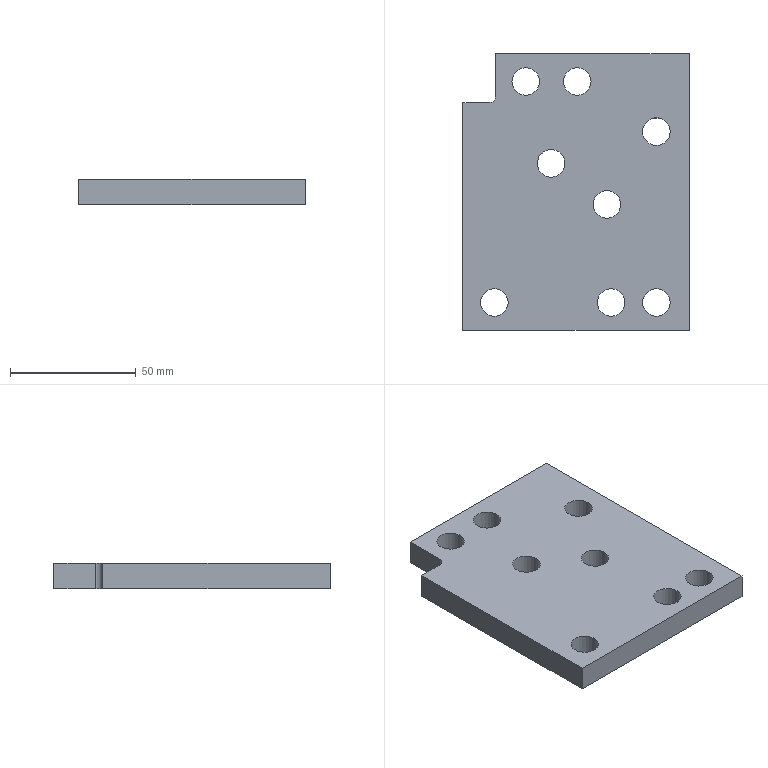Part | NX | features solid 2 | 1 solid | 17 faces | box 90 x 110 x 10 mm | volume 88862 mm3 | cylinder 9 | plane 8 | commonest cylinder face diameters 11 x8 6 x1
STEP:
#1=CARTESIAN_POINT('',(218.5,-15.984,78.));
#2=VERTEX_POINT('',#1);
#3=CARTESIAN_POINT('',(295.411,-15.984,78.));
#4=VERTEX_POINT('',#3);
#5=CARTESIAN_POINT('',(247.131,-15.984,78.));
#6=DIRECTION('',(1.,0.,0.));
#7=VECTOR('',#6,1000.);
#8=LINE('',#5,#7);
#9=EDGE_CURVE('',#2,#4,#8,.T.);
#10=ORIENTED_EDGE('',*,*,#9,.T.);
#11=CARTESIAN_POINT('',(295.411,-125.984,78.));
#12=VERTEX_POINT('',#11);
#13=CARTESIAN_POINT('',(295.411,-71.771,78.));
#14=DIRECTION('',(0.,-1.,0.));
#15=VECTOR('',#14,1000.);
#16=LINE('',#13,#15);
#17=EDGE_CURVE('',#4,#12,#16,.T.);
#18=ORIENTED_EDGE('',*,*,#17,.T.);
#19=CARTESIAN_POINT('',(205.411,-125.984,78.));
#20=VERTEX_POINT('',#19);
#21=CARTESIAN_POINT('',(247.131,-125.984,78.));
#22=DIRECTION('',(-1.,0.,0.));
#23=VECTOR('',#22,1000.);
#24=LINE('',#21,#23);
#25=EDGE_CURVE('',#12,#20,#24,.T.);
#26=ORIENTED_EDGE('',*,*,#25,.T.);
#27=CARTESIAN_POINT('',(205.411,-35.5,78.));
#28=VERTEX_POINT('',#27);
#29=CARTESIAN_POINT('',(205.411,-71.771,78.));
#30=DIRECTION('',(0.,1.,0.));
#31=VECTOR('',#30,1000.);
#32=LINE('',#29,#31);
#33=EDGE_CURVE('',#20,#28,#32,.T.);
#34=ORIENTED_EDGE('',*,*,#33,.T.);
#35=CARTESIAN_POINT('',(215.5,-35.5,78.));
#36=VERTEX_POINT('',#35);
#37=CARTESIAN_POINT('',(188.,-35.5,78.));
#38=DIRECTION('',(-1.,0.,0.));
#39=VECTOR('',#38,1000.);
#40=LINE('',#37,#39);
#41=EDGE_CURVE('',#28,#36,#40,.F.);
#42=ORIENTED_EDGE('',*,*,#41,.T.);
#43=CARTESIAN_POINT('',(218.5,-32.5,78.));
#44=VERTEX_POINT('',#43);
#45=CARTESIAN_POINT('',(215.5,-32.5,78.));
#46=DIRECTION('',(0.,0.,-1.));
#47=DIRECTION('',(-1.,0.,0.));
#48=AXIS2_PLACEMENT_3D('',#45,#46,#47);
#49=CIRCLE('',#48,3.);
#50=EDGE_CURVE('',#36,#44,#49,.F.);
#51=ORIENTED_EDGE('',*,*,#50,.T.);
#52=CARTESIAN_POINT('',(218.5,0.,78.));
#53=DIRECTION('',(0.,-1.,0.));
#54=VECTOR('',#53,1000.);
#55=LINE('',#52,#54);
#56=EDGE_CURVE('',#44,#2,#55,.F.);
#57=ORIENTED_EDGE('',*,*,#56,.T.);
#58=EDGE_LOOP('',(#10,#18,#26,#34,#42,#51,#57));
#59=FACE_BOUND('',#58,.T.);
#60=CARTESIAN_POINT('',(258.911,-114.984,78.));
#61=VERTEX_POINT('',#60);
#62=CARTESIAN_POINT('',(264.411,-114.984,78.));
#63=DIRECTION('',(0.,0.,1.));
#64=DIRECTION('',(-1.,0.,0.));
#65=AXIS2_PLACEMENT_3D('',#62,#63,#64);
#66=CIRCLE('',#65,5.5);
#67=EDGE_CURVE('',#61,#61,#66,.F.);
#68=ORIENTED_EDGE('',*,*,#67,.F.);
#69=EDGE_LOOP('',(#68));
#70=FACE_BOUND('',#69,.T.);
#71=CARTESIAN_POINT('',(276.911,-114.984,78.));
#72=VERTEX_POINT('',#71);
#73=CARTESIAN_POINT('',(282.411,-114.984,78.));
#74=DIRECTION('',(0.,0.,-1.));
#75=DIRECTION('',(-1.,0.,0.));
#76=AXIS2_PLACEMENT_3D('',#73,#74,#75);
#77=CIRCLE('',#76,5.5);
#78=EDGE_CURVE('',#72,#72,#77,.F.);
#79=ORIENTED_EDGE('',*,*,#78,.T.);
#80=EDGE_LOOP('',(#79));
#81=FACE_BOUND('',#80,.T.);
#82=CARTESIAN_POINT('',(224.911,-26.984,78.));
#83=VERTEX_POINT('',#82);
#84=CARTESIAN_POINT('',(230.411,-26.984,78.));
#85=DIRECTION('',(0.,0.,-1.));
#86=DIRECTION('',(-1.,0.,0.));
#87=AXIS2_PLACEMENT_3D('',#84,#85,#86);
#88=CIRCLE('',#87,5.5);
#89=EDGE_CURVE('',#83,#83,#88,.F.);
#90=ORIENTED_EDGE('',*,*,#89,.T.);
#91=EDGE_LOOP('',(#90));
#92=FACE_BOUND('',#91,.T.);
#93=CARTESIAN_POINT('',(276.911,-46.984,78.));
#94=VERTEX_POINT('',#93);
#95=CARTESIAN_POINT('',(282.411,-46.984,78.));
#96=DIRECTION('',(0.,0.,-1.));
#97=DIRECTION('',(-1.,0.,0.));
#98=AXIS2_PLACEMENT_3D('',#95,#96,#97);
#99=CIRCLE('',#98,5.5);
#100=EDGE_CURVE('',#94,#94,#99,.F.);
#101=ORIENTED_EDGE('',*,*,#100,.T.);
#102=EDGE_LOOP('',(#101));
#103=FACE_BOUND('',#102,.T.);
#104=CARTESIAN_POINT('',(212.411,-114.984,78.));
#105=VERTEX_POINT('',#104);
#106=CARTESIAN_POINT('',(217.911,-114.984,78.));
#107=DIRECTION('',(0.,0.,-1.));
#108=DIRECTION('',(-1.,0.,0.));
#109=AXIS2_PLACEMENT_3D('',#106,#107,#108);
#110=CIRCLE('',#109,5.5);
#111=EDGE_CURVE('',#105,#105,#110,.F.);
#112=ORIENTED_EDGE('',*,*,#111,.T.);
#113=EDGE_LOOP('',(#112));
#114=FACE_BOUND('',#113,.T.);
#115=CARTESIAN_POINT('',(245.411,-26.984,78.));
#116=VERTEX_POINT('',#115);
#117=CARTESIAN_POINT('',(250.911,-26.984,78.));
#118=DIRECTION('',(0.,0.,1.));
#119=DIRECTION('',(-1.,0.,0.));
#120=AXIS2_PLACEMENT_3D('',#117,#118,#119);
#121=CIRCLE('',#120,5.5);
#122=EDGE_CURVE('',#116,#116,#121,.T.);
#123=ORIENTED_EDGE('',*,*,#122,.T.);
#124=EDGE_LOOP('',(#123));
#125=FACE_BOUND('',#124,.T.);
#126=CARTESIAN_POINT('',(257.24,-75.929,78.));
#127=VERTEX_POINT('',#126);
#128=CARTESIAN_POINT('',(262.74,-75.929,78.));
#129=DIRECTION('',(0.,0.,1.));
#130=DIRECTION('',(-1.,0.,0.));
#131=AXIS2_PLACEMENT_3D('',#128,#129,#130);
#132=CIRCLE('',#131,5.5);
#133=EDGE_CURVE('',#127,#127,#132,.F.);
#134=ORIENTED_EDGE('',*,*,#133,.F.);
#135=EDGE_LOOP('',(#134));
#136=FACE_BOUND('',#135,.T.);
#137=CARTESIAN_POINT('',(235.001,-59.571,78.));
#138=VERTEX_POINT('',#137);
#139=CARTESIAN_POINT('',(240.501,-59.571,78.));
#140=DIRECTION('',(0.,0.,1.));
#141=DIRECTION('',(-1.,0.,0.));
#142=AXIS2_PLACEMENT_3D('',#139,#140,#141);
#143=CIRCLE('',#142,5.5);
#144=EDGE_CURVE('',#138,#138,#143,.T.);
#145=ORIENTED_EDGE('',*,*,#144,.T.);
#146=EDGE_LOOP('',(#145));
#147=FACE_BOUND('',#146,.T.);
#148=CARTESIAN_POINT('',(252.074,-71.771,78.));
#149=DIRECTION('',(0.,0.,-1.));
#150=DIRECTION('',(-1.,0.,0.));
#151=AXIS2_PLACEMENT_3D('',#148,#149,#150);
#152=PLANE('',#151);
#153=ADVANCED_FACE('',(#59,#70,#81,#92,#103,#114,#125,#136,#147),#152,.T.);
#154=ORIENTED_EDGE('',*,*,#144,.F.);
#155=EDGE_LOOP('',(#154));
#156=FACE_BOUND('',#155,.T.);
#157=CARTESIAN_POINT('',(235.001,-59.571,88.));
#158=VERTEX_POINT('',#157);
#159=CARTESIAN_POINT('',(240.501,-59.571,88.));
#160=DIRECTION('',(0.,0.,1.));
#161=DIRECTION('',(-1.,0.,0.));
#162=AXIS2_PLACEMENT_3D('',#159,#160,#161);
#163=CIRCLE('',#162,5.5);
#164=EDGE_CURVE('',#158,#158,#163,.T.);
#165=ORIENTED_EDGE('',*,*,#164,.T.);
#166=EDGE_LOOP('',(#165));
#167=FACE_BOUND('',#166,.T.);
#168=CARTESIAN_POINT('',(240.501,-59.571,78.));
#169=DIRECTION('',(0.,0.,-1.));
#170=DIRECTION('',(-1.,0.,0.));
#171=AXIS2_PLACEMENT_3D('',#168,#169,#170);
#172=CYLINDRICAL_SURFACE('',#171,5.5);
#173=ADVANCED_FACE('',(#156,#167),#172,.F.);
#174=CARTESIAN_POINT('',(224.911,-26.984,88.));
#175=VERTEX_POINT('',#174);
#176=CARTESIAN_POINT('',(230.411,-26.984,88.));
#177=DIRECTION('',(0.,0.,1.));
#178=DIRECTION('',(-1.,0.,0.));
#179=AXIS2_PLACEMENT_3D('',#176,#177,#178);
#180=CIRCLE('',#179,5.5);
#181=EDGE_CURVE('',#175,#175,#180,.F.);
#182=ORIENTED_EDGE('',*,*,#181,.F.);
#183=EDGE_LOOP('',(#182));
#184=FACE_BOUND('',#183,.T.);
#185=ORIENTED_EDGE('',*,*,#89,.F.);
#186=EDGE_LOOP('',(#185));
#187=FACE_BOUND('',#186,.T.);
#188=CARTESIAN_POINT('',(230.411,-26.984,78.));
#189=DIRECTION('',(0.,0.,-1.));
#190=DIRECTION('',(-1.,0.,0.));
#191=AXIS2_PLACEMENT_3D('',#188,#189,#190);
#192=CYLINDRICAL_SURFACE('',#191,5.5);
#193=ADVANCED_FACE('',(#184,#187),#192,.F.);
#194=CARTESIAN_POINT('',(276.911,-46.984,88.));
#195=VERTEX_POINT('',#194);
#196=CARTESIAN_POINT('',(282.411,-46.984,88.));
#197=DIRECTION('',(0.,0.,1.));
#198=DIRECTION('',(-1.,0.,0.));
#199=AXIS2_PLACEMENT_3D('',#196,#197,#198);
#200=CIRCLE('',#199,5.5);
#201=EDGE_CURVE('',#195,#195,#200,.F.);
#202=ORIENTED_EDGE('',*,*,#201,.F.);
#203=EDGE_LOOP('',(#202));
#204=FACE_BOUND('',#203,.T.);
#205=ORIENTED_EDGE('',*,*,#100,.F.);
#206=EDGE_LOOP('',(#205));
#207=FACE_BOUND('',#206,.T.);
#208=CARTESIAN_POINT('',(282.411,-46.984,78.));
#209=DIRECTION('',(0.,0.,-1.));
#210=DIRECTION('',(-1.,0.,0.));
#211=AXIS2_PLACEMENT_3D('',#208,#209,#210);
#212=CYLINDRICAL_SURFACE('',#211,5.5);
#213=ADVANCED_FACE('',(#204,#207),#212,.F.);
#214=CARTESIAN_POINT('',(276.911,-114.984,88.));
#215=VERTEX_POINT('',#214);
#216=CARTESIAN_POINT('',(282.411,-114.984,88.));
#217=DIRECTION('',(0.,0.,1.));
#218=DIRECTION('',(-1.,0.,0.));
#219=AXIS2_PLACEMENT_3D('',#216,#217,#218);
#220=CIRCLE('',#219,5.5);
#221=EDGE_CURVE('',#215,#215,#220,.T.);
#222=ORIENTED_EDGE('',*,*,#221,.T.);
#223=EDGE_LOOP('',(#222));
#224=FACE_BOUND('',#223,.T.);
#225=ORIENTED_EDGE('',*,*,#78,.F.);
#226=EDGE_LOOP('',(#225));
#227=FACE_BOUND('',#226,.T.);
#228=CARTESIAN_POINT('',(282.411,-114.984,78.));
#229=DIRECTION('',(0.,0.,-1.));
#230=DIRECTION('',(-1.,0.,0.));
#231=AXIS2_PLACEMENT_3D('',#228,#229,#230);
#232=CYLINDRICAL_SURFACE('',#231,5.5);
#233=ADVANCED_FACE('',(#224,#227),#232,.F.);
#234=CARTESIAN_POINT('',(212.411,-114.984,88.));
#235=VERTEX_POINT('',#234);
#236=CARTESIAN_POINT('',(217.911,-114.984,88.));
#237=DIRECTION('',(0.,0.,1.));
#238=DIRECTION('',(-1.,0.,0.));
#239=AXIS2_PLACEMENT_3D('',#236,#237,#238);
#240=CIRCLE('',#239,5.5);
#241=EDGE_CURVE('',#235,#235,#240,.T.);
#242=ORIENTED_EDGE('',*,*,#241,.T.);
#243=EDGE_LOOP('',(#242));
#244=FACE_BOUND('',#243,.T.);
#245=ORIENTED_EDGE('',*,*,#111,.F.);
#246=EDGE_LOOP('',(#245));
#247=FACE_BOUND('',#246,.T.);
#248=CARTESIAN_POINT('',(217.911,-114.984,78.));
#249=DIRECTION('',(0.,0.,-1.));
#250=DIRECTION('',(-1.,0.,0.));
#251=AXIS2_PLACEMENT_3D('',#248,#249,#250);
#252=CYLINDRICAL_SURFACE('',#251,5.5);
#253=ADVANCED_FACE('',(#244,#247),#252,.F.);
#254=ORIENTED_EDGE('',*,*,#67,.T.);
#255=EDGE_LOOP('',(#254));
#256=FACE_BOUND('',#255,.T.);
#257=CARTESIAN_POINT('',(258.911,-114.984,88.));
#258=VERTEX_POINT('',#257);
#259=CARTESIAN_POINT('',(264.411,-114.984,88.));
#260=DIRECTION('',(0.,0.,1.));
#261=DIRECTION('',(-1.,0.,0.));
#262=AXIS2_PLACEMENT_3D('',#259,#260,#261);
#263=CIRCLE('',#262,5.5);
#264=EDGE_CURVE('',#258,#258,#263,.F.);
#265=ORIENTED_EDGE('',*,*,#264,.F.);
#266=EDGE_LOOP('',(#265));
#267=FACE_BOUND('',#266,.T.);
#268=CARTESIAN_POINT('',(264.411,-114.984,78.));
#269=DIRECTION('',(0.,0.,-1.));
#270=DIRECTION('',(-1.,0.,0.));
#271=AXIS2_PLACEMENT_3D('',#268,#269,#270);
#272=CYLINDRICAL_SURFACE('',#271,5.5);
#273=ADVANCED_FACE('',(#256,#267),#272,.F.);
#274=ORIENTED_EDGE('',*,*,#122,.F.);
#275=EDGE_LOOP('',(#274));
#276=FACE_BOUND('',#275,.T.);
#277=CARTESIAN_POINT('',(245.411,-26.984,88.));
#278=VERTEX_POINT('',#277);
#279=CARTESIAN_POINT('',(250.911,-26.984,88.));
#280=DIRECTION('',(0.,0.,1.));
#281=DIRECTION('',(-1.,0.,0.));
#282=AXIS2_PLACEMENT_3D('',#279,#280,#281);
#283=CIRCLE('',#282,5.5);
#284=EDGE_CURVE('',#278,#278,#283,.T.);
#285=ORIENTED_EDGE('',*,*,#284,.T.);
#286=EDGE_LOOP('',(#285));
#287=FACE_BOUND('',#286,.T.);
#288=CARTESIAN_POINT('',(250.911,-26.984,78.));
#289=DIRECTION('',(0.,0.,-1.));
#290=DIRECTION('',(-1.,0.,0.));
#291=AXIS2_PLACEMENT_3D('',#288,#289,#290);
#292=CYLINDRICAL_SURFACE('',#291,5.5);
#293=ADVANCED_FACE('',(#276,#287),#292,.F.);
#294=CARTESIAN_POINT('',(295.411,-125.984,88.));
#295=VERTEX_POINT('',#294);
#296=CARTESIAN_POINT('',(295.411,-15.984,88.));
#297=VERTEX_POINT('',#296);
#298=CARTESIAN_POINT('',(295.411,-71.771,88.));
#299=DIRECTION('',(0.,-1.,0.));
#300=VECTOR('',#299,1000.);
#301=LINE('',#298,#300);
#302=EDGE_CURVE('',#295,#297,#301,.F.);
#303=ORIENTED_EDGE('',*,*,#302,.T.);
#304=CARTESIAN_POINT('',(218.5,-15.984,88.));
#305=VERTEX_POINT('',#304);
#306=CARTESIAN_POINT('',(188.,-15.984,88.));
#307=DIRECTION('',(-1.,0.,0.));
#308=VECTOR('',#307,1000.);
#309=LINE('',#306,#308);
#310=EDGE_CURVE('',#297,#305,#309,.T.);
#311=ORIENTED_EDGE('',*,*,#310,.T.);
#312=CARTESIAN_POINT('',(218.5,-32.5,88.));
#313=VERTEX_POINT('',#312);
#314=CARTESIAN_POINT('',(218.5,0.,88.));
#315=DIRECTION('',(0.,-1.,0.));
#316=VECTOR('',#315,1000.);
#317=LINE('',#314,#316);
#318=EDGE_CURVE('',#305,#313,#317,.T.);
#319=ORIENTED_EDGE('',*,*,#318,.T.);
#320=CARTESIAN_POINT('',(215.5,-35.5,88.));
#321=VERTEX_POINT('',#320);
#322=CARTESIAN_POINT('',(215.5,-32.5,88.));
#323=DIRECTION('',(0.,0.,-1.));
#324=DIRECTION('',(-1.,0.,0.));
#325=AXIS2_PLACEMENT_3D('',#322,#323,#324);
#326=CIRCLE('',#325,3.);
#327=EDGE_CURVE('',#313,#321,#326,.T.);
#328=ORIENTED_EDGE('',*,*,#327,.T.);
#329=CARTESIAN_POINT('',(205.411,-35.5,88.));
#330=VERTEX_POINT('',#329);
#331=CARTESIAN_POINT('',(188.,-35.5,88.));
#332=DIRECTION('',(-1.,0.,0.));
#333=VECTOR('',#332,1000.);
#334=LINE('',#331,#333);
#335=EDGE_CURVE('',#321,#330,#334,.T.);
#336=ORIENTED_EDGE('',*,*,#335,.T.);
#337=CARTESIAN_POINT('',(205.411,-125.984,88.));
#338=VERTEX_POINT('',#337);
#339=CARTESIAN_POINT('',(205.411,0.,88.));
#340=DIRECTION('',(0.,-1.,0.));
#341=VECTOR('',#340,1000.);
#342=LINE('',#339,#341);
#343=EDGE_CURVE('',#330,#338,#342,.T.);
#344=ORIENTED_EDGE('',*,*,#343,.T.);
#345=CARTESIAN_POINT('',(188.,-125.984,88.));
#346=DIRECTION('',(-1.,0.,0.));
#347=VECTOR('',#346,1000.);
#348=LINE('',#345,#347);
#349=EDGE_CURVE('',#338,#295,#348,.F.);
#350=ORIENTED_EDGE('',*,*,#349,.T.);
#351=EDGE_LOOP('',(#303,#311,#319,#328,#336,#344,#350));
#352=FACE_BOUND('',#351,.T.);
#353=CARTESIAN_POINT('',(257.24,-75.929,88.));
#354=VERTEX_POINT('',#353);
#355=CARTESIAN_POINT('',(262.74,-75.929,88.));
#356=DIRECTION('',(0.,0.,1.));
#357=DIRECTION('',(-1.,0.,0.));
#358=AXIS2_PLACEMENT_3D('',#355,#356,#357);
#359=CIRCLE('',#358,5.5);
#360=EDGE_CURVE('',#354,#354,#359,.F.);
#361=ORIENTED_EDGE('',*,*,#360,.T.);
#362=EDGE_LOOP('',(#361));
#363=FACE_BOUND('',#362,.T.);
#364=ORIENTED_EDGE('',*,*,#164,.F.);
#365=EDGE_LOOP('',(#364));
#366=FACE_BOUND('',#365,.T.);
#367=ORIENTED_EDGE('',*,*,#284,.F.);
#368=EDGE_LOOP('',(#367));
#369=FACE_BOUND('',#368,.T.);
#370=ORIENTED_EDGE('',*,*,#264,.T.);
#371=EDGE_LOOP('',(#370));
#372=FACE_BOUND('',#371,.T.);
#373=ORIENTED_EDGE('',*,*,#241,.F.);
#374=EDGE_LOOP('',(#373));
#375=FACE_BOUND('',#374,.T.);
#376=ORIENTED_EDGE('',*,*,#221,.F.);
#377=EDGE_LOOP('',(#376));
#378=FACE_BOUND('',#377,.T.);
#379=ORIENTED_EDGE('',*,*,#201,.T.);
#380=EDGE_LOOP('',(#379));
#381=FACE_BOUND('',#380,.T.);
#382=ORIENTED_EDGE('',*,*,#181,.T.);
#383=EDGE_LOOP('',(#382));
#384=FACE_BOUND('',#383,.T.);
#385=CARTESIAN_POINT('',(188.,0.,88.));
#386=DIRECTION('',(0.,0.,-1.));
#387=DIRECTION('',(-1.,0.,0.));
#388=AXIS2_PLACEMENT_3D('',#385,#386,#387);
#389=PLANE('',#388);
#390=ADVANCED_FACE('',(#352,#363,#366,#369,#372,#375,#378,#381,#384),#389,.F.);
#391=ORIENTED_EDGE('',*,*,#310,.F.);
#392=CARTESIAN_POINT('',(295.411,-15.984,78.));
#393=DIRECTION('',(0.,0.,1.));
#394=VECTOR('',#393,1000.);
#395=LINE('',#392,#394);
#396=EDGE_CURVE('',#297,#4,#395,.F.);
#397=ORIENTED_EDGE('',*,*,#396,.T.);
#398=ORIENTED_EDGE('',*,*,#9,.F.);
#399=CARTESIAN_POINT('',(218.5,-15.984,78.));
#400=DIRECTION('',(0.,0.,1.));
#401=VECTOR('',#400,1000.);
#402=LINE('',#399,#401);
#403=EDGE_CURVE('',#2,#305,#402,.T.);
#404=ORIENTED_EDGE('',*,*,#403,.T.);
#405=EDGE_LOOP('',(#391,#397,#398,#404));
#406=FACE_BOUND('',#405,.T.);
#407=CARTESIAN_POINT('',(247.131,-15.984,78.));
#408=DIRECTION('',(0.,-1.,0.));
#409=DIRECTION('',(1.,0.,0.));
#410=AXIS2_PLACEMENT_3D('',#407,#408,#409);
#411=PLANE('',#410);
#412=ADVANCED_FACE('',(#406),#411,.F.);
#413=ORIENTED_EDGE('',*,*,#56,.F.);
#414=CARTESIAN_POINT('',(218.5,-32.5,88.));
#415=DIRECTION('',(0.,0.,-1.));
#416=VECTOR('',#415,1000.);
#417=LINE('',#414,#416);
#418=EDGE_CURVE('',#44,#313,#417,.F.);
#419=ORIENTED_EDGE('',*,*,#418,.T.);
#420=ORIENTED_EDGE('',*,*,#318,.F.);
#421=ORIENTED_EDGE('',*,*,#403,.F.);
#422=EDGE_LOOP('',(#413,#419,#420,#421));
#423=FACE_BOUND('',#422,.T.);
#424=CARTESIAN_POINT('',(218.5,0.,78.));
#425=DIRECTION('',(-1.,0.,0.));
#426=DIRECTION('',(0.,-1.,0.));
#427=AXIS2_PLACEMENT_3D('',#424,#425,#426);
#428=PLANE('',#427);
#429=ADVANCED_FACE('',(#423),#428,.T.);
#430=ORIENTED_EDGE('',*,*,#335,.F.);
#431=CARTESIAN_POINT('',(215.5,-35.5,78.));
#432=DIRECTION('',(0.,0.,-1.));
#433=VECTOR('',#432,1000.);
#434=LINE('',#431,#433);
#435=EDGE_CURVE('',#321,#36,#434,.T.);
#436=ORIENTED_EDGE('',*,*,#435,.T.);
#437=ORIENTED_EDGE('',*,*,#41,.F.);
#438=CARTESIAN_POINT('',(205.411,-35.5,78.));
#439=DIRECTION('',(0.,0.,1.));
#440=VECTOR('',#439,1000.);
#441=LINE('',#438,#440);
#442=EDGE_CURVE('',#330,#28,#441,.F.);
#443=ORIENTED_EDGE('',*,*,#442,.F.);
#444=EDGE_LOOP('',(#430,#436,#437,#443));
#445=FACE_BOUND('',#444,.T.);
#446=CARTESIAN_POINT('',(188.,-35.5,78.));
#447=DIRECTION('',(0.,1.,0.));
#448=DIRECTION('',(-1.,0.,0.));
#449=AXIS2_PLACEMENT_3D('',#446,#447,#448);
#450=PLANE('',#449);
#451=ADVANCED_FACE('',(#445),#450,.T.);
#452=ORIENTED_EDGE('',*,*,#33,.F.);
#453=CARTESIAN_POINT('',(205.411,-125.984,78.));
#454=DIRECTION('',(0.,0.,1.));
#455=VECTOR('',#454,1000.);
#456=LINE('',#453,#455);
#457=EDGE_CURVE('',#20,#338,#456,.T.);
#458=ORIENTED_EDGE('',*,*,#457,.T.);
#459=ORIENTED_EDGE('',*,*,#343,.F.);
#460=ORIENTED_EDGE('',*,*,#442,.T.);
#461=EDGE_LOOP('',(#452,#458,#459,#460));
#462=FACE_BOUND('',#461,.T.);
#463=CARTESIAN_POINT('',(205.411,-71.771,78.));
#464=DIRECTION('',(1.,0.,0.));
#465=DIRECTION('',(0.,1.,0.));
#466=AXIS2_PLACEMENT_3D('',#463,#464,#465);
#467=PLANE('',#466);
#468=ADVANCED_FACE('',(#462),#467,.F.);
#469=ORIENTED_EDGE('',*,*,#25,.F.);
#470=CARTESIAN_POINT('',(295.411,-125.984,78.));
#471=DIRECTION('',(0.,0.,-1.));
#472=VECTOR('',#471,1000.);
#473=LINE('',#470,#472);
#474=EDGE_CURVE('',#12,#295,#473,.F.);
#475=ORIENTED_EDGE('',*,*,#474,.T.);
#476=ORIENTED_EDGE('',*,*,#349,.F.);
#477=ORIENTED_EDGE('',*,*,#457,.F.);
#478=EDGE_LOOP('',(#469,#475,#476,#477));
#479=FACE_BOUND('',#478,.T.);
#480=CARTESIAN_POINT('',(247.131,-125.984,78.));
#481=DIRECTION('',(0.,1.,0.));
#482=DIRECTION('',(-1.,0.,0.));
#483=AXIS2_PLACEMENT_3D('',#480,#481,#482);
#484=PLANE('',#483);
#485=ADVANCED_FACE('',(#479),#484,.F.);
#486=ORIENTED_EDGE('',*,*,#17,.F.);
#487=ORIENTED_EDGE('',*,*,#396,.F.);
#488=ORIENTED_EDGE('',*,*,#302,.F.);
#489=ORIENTED_EDGE('',*,*,#474,.F.);
#490=EDGE_LOOP('',(#486,#487,#488,#489));
#491=FACE_BOUND('',#490,.T.);
#492=CARTESIAN_POINT('',(295.411,-71.771,78.));
#493=DIRECTION('',(-1.,0.,0.));
#494=DIRECTION('',(0.,-1.,0.));
#495=AXIS2_PLACEMENT_3D('',#492,#493,#494);
#496=PLANE('',#495);
#497=ADVANCED_FACE('',(#491),#496,.F.);
#498=ORIENTED_EDGE('',*,*,#133,.T.);
#499=EDGE_LOOP('',(#498));
#500=FACE_BOUND('',#499,.T.);
#501=ORIENTED_EDGE('',*,*,#360,.F.);
#502=EDGE_LOOP('',(#501));
#503=FACE_BOUND('',#502,.T.);
#504=CARTESIAN_POINT('',(262.74,-75.929,78.));
#505=DIRECTION('',(0.,0.,-1.));
#506=DIRECTION('',(-1.,0.,0.));
#507=AXIS2_PLACEMENT_3D('',#504,#505,#506);
#508=CYLINDRICAL_SURFACE('',#507,5.5);
#509=ADVANCED_FACE('',(#500,#503),#508,.F.);
#510=ORIENTED_EDGE('',*,*,#50,.F.);
#511=ORIENTED_EDGE('',*,*,#435,.F.);
#512=ORIENTED_EDGE('',*,*,#327,.F.);
#513=ORIENTED_EDGE('',*,*,#418,.F.);
#514=EDGE_LOOP('',(#510,#511,#512,#513));
#515=FACE_BOUND('',#514,.T.);
#516=CARTESIAN_POINT('',(215.5,-32.5,78.));
#517=DIRECTION('',(0.,0.,-1.));
#518=DIRECTION('',(-1.,0.,0.));
#519=AXIS2_PLACEMENT_3D('',#516,#517,#518);
#520=CYLINDRICAL_SURFACE('',#519,3.);
#521=ADVANCED_FACE('',(#515),#520,.F.);
#522=CLOSED_SHELL('',(#153,#173,#193,#213,#233,#253,#273,#293,#390,#412,#429,#451,#468,#485,#497,#509,#521));
#523=MANIFOLD_SOLID_BREP('',#522);
#524=(LENGTH_UNIT()NAMED_UNIT(*)SI_UNIT(.MILLI.,.METRE.));
#525=UNCERTAINTY_MEASURE_WITH_UNIT(LENGTH_MEASURE(0.00001),#524,'','');
#526=(NAMED_UNIT(*)PLANE_ANGLE_UNIT()SI_UNIT($,.RADIAN.));
#527=(NAMED_UNIT(*)SI_UNIT($,.STERADIAN.)SOLID_ANGLE_UNIT());
#528=(GEOMETRIC_REPRESENTATION_CONTEXT(3)GLOBAL_UNCERTAINTY_ASSIGNED_CONTEXT((#525))GLOBAL_UNIT_ASSIGNED_CONTEXT((#524,#526,#527))REPRESENTATION_CONTEXT('',''));
#529=ADVANCED_BREP_SHAPE_REPRESENTATION('',(#523),#528);